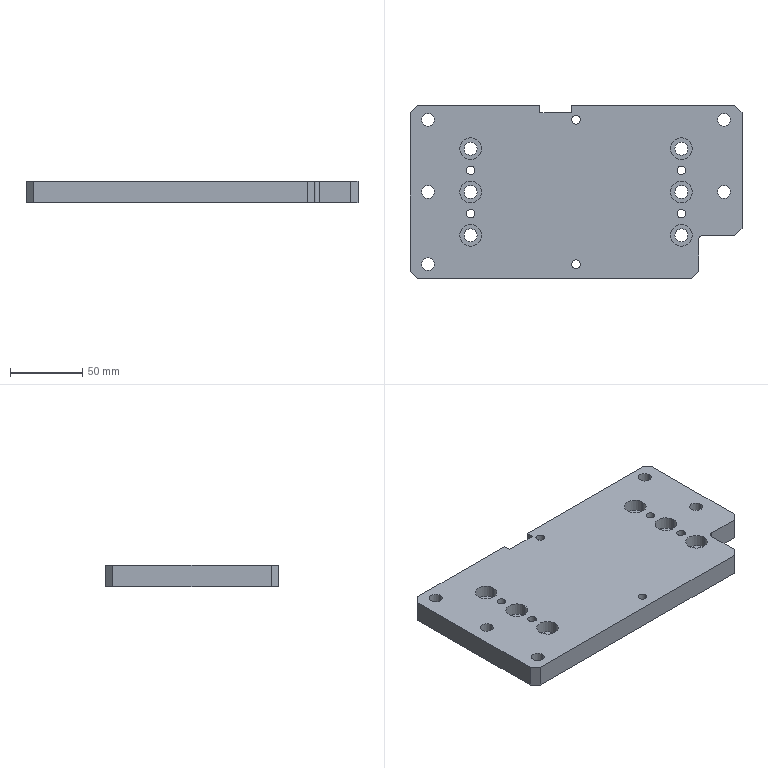Part | STEP file | PN_0012 | 1 solid | 93 faces | box 230 x 120 x 15 mm | volume 374023 mm3 | cylinder 61 | plane 28 | cone 4 | commonest cylinder face diameters 9 x22 15 x22 6 x13 3.3 x4